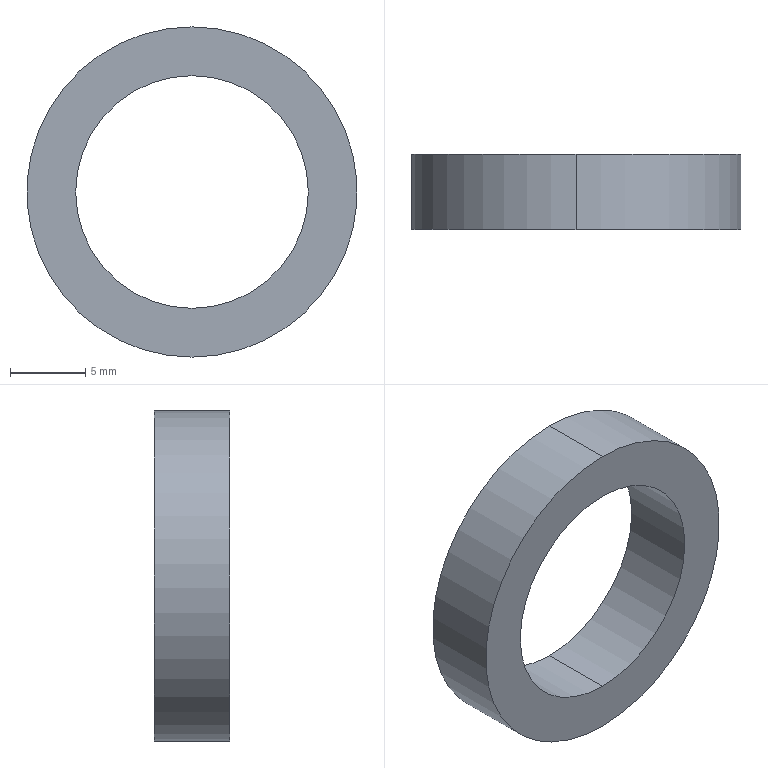Part | SolidWorks | features Extrusion 1, HoleWzd 1 | 1 solid | 6 faces | box 22 x 5 x 22 mm | volume 957.204 mm3 | cylinder 4 | plane 2 | commonest cylinder face diameters 15.5 x2 22 x2
STEP:
#1=CARTESIAN_POINT('',(0.,0.,-7.75));
#2=VERTEX_POINT('',#1);
#3=CARTESIAN_POINT('',(0.,0.,7.75));
#4=VERTEX_POINT('',#3);
#5=CARTESIAN_POINT('',(0.,0.,0.));
#6=DIRECTION('',(0.,1.,0.));
#7=DIRECTION('',(0.,0.,1.));
#8=AXIS2_PLACEMENT_3D('',#5,#6,#7);
#9=CIRCLE('',#8,7.75);
#10=EDGE_CURVE('',#2,#4,#9,.T.);
#11=ORIENTED_EDGE('',*,*,#10,.F.);
#12=CARTESIAN_POINT('',(0.,5.,-7.75));
#13=VERTEX_POINT('',#12);
#14=CARTESIAN_POINT('',(0.,5.,-7.75));
#15=DIRECTION('',(0.,1.,0.));
#16=VECTOR('',#15,1000.);
#17=LINE('',#14,#16);
#18=EDGE_CURVE('',#2,#13,#17,.T.);
#19=ORIENTED_EDGE('',*,*,#18,.T.);
#20=CARTESIAN_POINT('',(0.,5.,7.75));
#21=VERTEX_POINT('',#20);
#22=CARTESIAN_POINT('',(0.,5.,0.));
#23=DIRECTION('',(0.,1.,0.));
#24=DIRECTION('',(0.,0.,1.));
#25=AXIS2_PLACEMENT_3D('',#22,#23,#24);
#26=CIRCLE('',#25,7.75);
#27=EDGE_CURVE('',#13,#21,#26,.T.);
#28=ORIENTED_EDGE('',*,*,#27,.T.);
#29=CARTESIAN_POINT('',(0.,5.,7.75));
#30=DIRECTION('',(0.,1.,0.));
#31=VECTOR('',#30,1000.);
#32=LINE('',#29,#31);
#33=EDGE_CURVE('',#4,#21,#32,.T.);
#34=ORIENTED_EDGE('',*,*,#33,.F.);
#35=EDGE_LOOP('',(#11,#19,#28,#34));
#36=FACE_OUTER_BOUND('',#35,.T.);
#37=CARTESIAN_POINT('',(0.,5.,0.));
#38=DIRECTION('',(0.,1.,0.));
#39=DIRECTION('',(0.,0.,1.));
#40=AXIS2_PLACEMENT_3D('',#37,#38,#39);
#41=CYLINDRICAL_SURFACE('',#40,7.75);
#42=ADVANCED_FACE('',(#36),#41,.F.);
#43=CARTESIAN_POINT('',(0.,5.,11.));
#44=VERTEX_POINT('',#43);
#45=CARTESIAN_POINT('',(0.,5.,-11.));
#46=VERTEX_POINT('',#45);
#47=CARTESIAN_POINT('',(0.,5.,0.));
#48=DIRECTION('',(0.,1.,0.));
#49=DIRECTION('',(0.,0.,1.));
#50=AXIS2_PLACEMENT_3D('',#47,#48,#49);
#51=CIRCLE('',#50,11.);
#52=EDGE_CURVE('',#44,#46,#51,.T.);
#53=ORIENTED_EDGE('',*,*,#52,.F.);
#54=CARTESIAN_POINT('',(0.,0.,11.));
#55=VERTEX_POINT('',#54);
#56=CARTESIAN_POINT('',(0.,5.,11.));
#57=DIRECTION('',(0.,-1.,0.));
#58=VECTOR('',#57,1000.);
#59=LINE('',#56,#58);
#60=EDGE_CURVE('',#44,#55,#59,.T.);
#61=ORIENTED_EDGE('',*,*,#60,.T.);
#62=CARTESIAN_POINT('',(0.,0.,-11.));
#63=VERTEX_POINT('',#62);
#64=CARTESIAN_POINT('',(0.,0.,0.));
#65=DIRECTION('',(0.,1.,0.));
#66=DIRECTION('',(0.,0.,1.));
#67=AXIS2_PLACEMENT_3D('',#64,#65,#66);
#68=CIRCLE('',#67,11.);
#69=EDGE_CURVE('',#55,#63,#68,.T.);
#70=ORIENTED_EDGE('',*,*,#69,.T.);
#71=CARTESIAN_POINT('',(0.,5.,-11.));
#72=DIRECTION('',(0.,-1.,0.));
#73=VECTOR('',#72,1000.);
#74=LINE('',#71,#73);
#75=EDGE_CURVE('',#46,#63,#74,.T.);
#76=ORIENTED_EDGE('',*,*,#75,.F.);
#77=EDGE_LOOP('',(#53,#61,#70,#76));
#78=FACE_OUTER_BOUND('',#77,.T.);
#79=CARTESIAN_POINT('',(0.,5.,0.));
#80=DIRECTION('',(0.,-1.,0.));
#81=DIRECTION('',(0.,0.,-1.));
#82=AXIS2_PLACEMENT_3D('',#79,#80,#81);
#83=CYLINDRICAL_SURFACE('',#82,11.);
#84=ADVANCED_FACE('',(#78),#83,.T.);
#85=ORIENTED_EDGE('',*,*,#60,.F.);
#86=CARTESIAN_POINT('',(0.,5.,0.));
#87=DIRECTION('',(0.,1.,0.));
#88=DIRECTION('',(0.,0.,1.));
#89=AXIS2_PLACEMENT_3D('',#86,#87,#88);
#90=CIRCLE('',#89,11.);
#91=EDGE_CURVE('',#46,#44,#90,.T.);
#92=ORIENTED_EDGE('',*,*,#91,.F.);
#93=ORIENTED_EDGE('',*,*,#75,.T.);
#94=CARTESIAN_POINT('',(0.,0.,0.));
#95=DIRECTION('',(0.,1.,0.));
#96=DIRECTION('',(0.,0.,1.));
#97=AXIS2_PLACEMENT_3D('',#94,#95,#96);
#98=CIRCLE('',#97,11.);
#99=EDGE_CURVE('',#63,#55,#98,.T.);
#100=ORIENTED_EDGE('',*,*,#99,.T.);
#101=EDGE_LOOP('',(#85,#92,#93,#100));
#102=FACE_OUTER_BOUND('',#101,.T.);
#103=CARTESIAN_POINT('',(0.,5.,0.));
#104=DIRECTION('',(0.,-1.,0.));
#105=DIRECTION('',(0.,0.,-1.));
#106=AXIS2_PLACEMENT_3D('',#103,#104,#105);
#107=CYLINDRICAL_SURFACE('',#106,11.);
#108=ADVANCED_FACE('',(#102),#107,.T.);
#109=CARTESIAN_POINT('',(0.,5.,0.));
#110=DIRECTION('',(0.,1.,0.));
#111=DIRECTION('',(0.,0.,1.));
#112=AXIS2_PLACEMENT_3D('',#109,#110,#111);
#113=CIRCLE('',#112,7.75);
#114=EDGE_CURVE('',#21,#13,#113,.T.);
#115=ORIENTED_EDGE('',*,*,#114,.F.);
#116=ORIENTED_EDGE('',*,*,#27,.F.);
#117=EDGE_LOOP('',(#115,#116));
#118=FACE_BOUND('',#117,.T.);
#119=ORIENTED_EDGE('',*,*,#91,.T.);
#120=ORIENTED_EDGE('',*,*,#52,.T.);
#121=EDGE_LOOP('',(#119,#120));
#122=FACE_OUTER_BOUND('',#121,.T.);
#123=CARTESIAN_POINT('',(0.,5.,0.));
#124=DIRECTION('',(0.,1.,0.));
#125=DIRECTION('',(0.,0.,1.));
#126=AXIS2_PLACEMENT_3D('',#123,#124,#125);
#127=PLANE('',#126);
#128=ADVANCED_FACE('',(#118,#122),#127,.T.);
#129=CARTESIAN_POINT('',(0.,0.,0.));
#130=DIRECTION('',(0.,1.,0.));
#131=DIRECTION('',(0.,0.,1.));
#132=AXIS2_PLACEMENT_3D('',#129,#130,#131);
#133=CIRCLE('',#132,7.75);
#134=EDGE_CURVE('',#4,#2,#133,.T.);
#135=ORIENTED_EDGE('',*,*,#134,.T.);
#136=ORIENTED_EDGE('',*,*,#10,.T.);
#137=EDGE_LOOP('',(#135,#136));
#138=FACE_BOUND('',#137,.T.);
#139=ORIENTED_EDGE('',*,*,#99,.F.);
#140=ORIENTED_EDGE('',*,*,#69,.F.);
#141=EDGE_LOOP('',(#139,#140));
#142=FACE_OUTER_BOUND('',#141,.T.);
#143=CARTESIAN_POINT('',(0.,0.,0.));
#144=DIRECTION('',(0.,1.,0.));
#145=DIRECTION('',(0.,0.,1.));
#146=AXIS2_PLACEMENT_3D('',#143,#144,#145);
#147=PLANE('',#146);
#148=ADVANCED_FACE('',(#138,#142),#147,.F.);
#149=ORIENTED_EDGE('',*,*,#18,.F.);
#150=ORIENTED_EDGE('',*,*,#134,.F.);
#151=ORIENTED_EDGE('',*,*,#33,.T.);
#152=ORIENTED_EDGE('',*,*,#114,.T.);
#153=EDGE_LOOP('',(#149,#150,#151,#152));
#154=FACE_OUTER_BOUND('',#153,.T.);
#155=CARTESIAN_POINT('',(0.,5.,0.));
#156=DIRECTION('',(0.,1.,0.));
#157=DIRECTION('',(0.,0.,1.));
#158=AXIS2_PLACEMENT_3D('',#155,#156,#157);
#159=CYLINDRICAL_SURFACE('',#158,7.75);
#160=ADVANCED_FACE('',(#154),#159,.F.);
#161=CLOSED_SHELL('',(#42,#84,#108,#128,#148,#160));
#162=MANIFOLD_SOLID_BREP('',#161);
#163=CARTESIAN_POINT('',(0.,0.,0.));
#164=DIRECTION('',(0.,0.,1.));
#165=DIRECTION('',(1.,0.,0.));
#166=AXIS2_PLACEMENT_3D('',#163,#164,#165);
#167=(LENGTH_UNIT()NAMED_UNIT(*)SI_UNIT(.MILLI.,.METRE.));
#168=UNCERTAINTY_MEASURE_WITH_UNIT(LENGTH_MEASURE(0.00001),#167,'','');
#169=(NAMED_UNIT(*)PLANE_ANGLE_UNIT()SI_UNIT($,.RADIAN.));
#170=(NAMED_UNIT(*)SI_UNIT($,.STERADIAN.)SOLID_ANGLE_UNIT());
#171=(GEOMETRIC_REPRESENTATION_CONTEXT(3)GLOBAL_UNCERTAINTY_ASSIGNED_CONTEXT((#168))GLOBAL_UNIT_ASSIGNED_CONTEXT((#167,#169,#170))REPRESENTATION_CONTEXT('',''));
#172=ADVANCED_BREP_SHAPE_REPRESENTATION('',(#162,#166),#171);